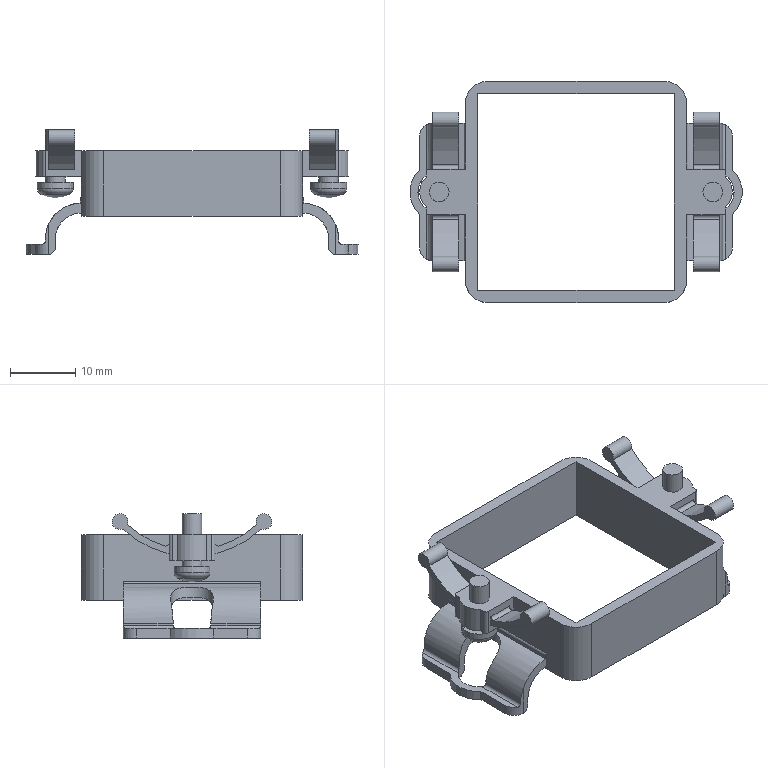Part | NX | 1 solid | 112 faces | box 50.8 x 33.8 x 19.002 mm | volume 3518 mm3 | plane 54 | cylinder 54 | sphere 2 | torus 2 | commonest cylinder face diameters 1 x14 2 x4 2.4 x4 3 x4 4 x4 6.8 x4